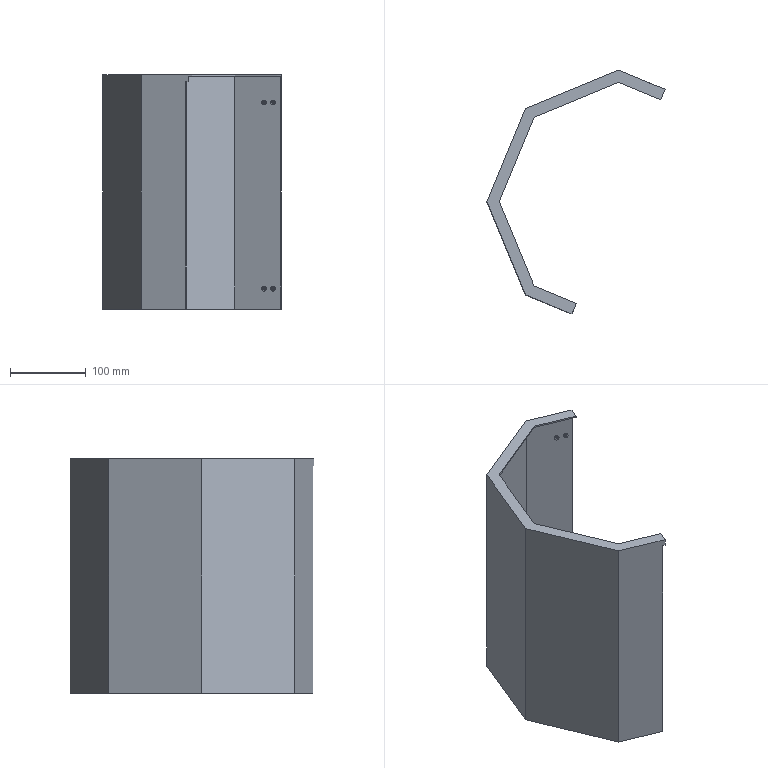Part | SolidWorks | features ICE 4, Extrusion 1, HoleWzd 1, RefAxis 1, Shell 1 | 1 solid | 42 faces | box 235.877 x 323.01 x 310 mm | volume 339899 mm3 | plane 26 | cylinder 16 | commonest cylinder face diameters 2.5 x8 6 x8
STEP:
#1=CARTESIAN_POINT('',(37.476,154.412,26.75));
#2=VERTEX_POINT('',#1);
#3=CARTESIAN_POINT('',(39.786,153.456,26.75));
#4=VERTEX_POINT('',#3);
#5=CARTESIAN_POINT('',(38.631,153.934,26.75));
#6=DIRECTION('',(-0.3827,-0.9239,0.));
#7=DIRECTION('',(0.9239,-0.3827,0.));
#8=AXIS2_PLACEMENT_3D('',#5,#6,#7);
#9=CIRCLE('',#8,1.25);
#10=EDGE_CURVE('',#2,#4,#9,.T.);
#11=ORIENTED_EDGE('',*,*,#10,.T.);
#12=CARTESIAN_POINT('',(41.317,157.151,26.75));
#13=VERTEX_POINT('',#12);
#14=CARTESIAN_POINT('',(41.317,157.151,26.75));
#15=DIRECTION('',(0.3827,0.9239,0.));
#16=VECTOR('',#15,1000.);
#17=LINE('',#14,#16);
#18=EDGE_CURVE('',#4,#13,#17,.T.);
#19=ORIENTED_EDGE('',*,*,#18,.T.);
#20=CARTESIAN_POINT('',(39.007,158.108,26.75));
#21=VERTEX_POINT('',#20);
#22=CARTESIAN_POINT('',(40.162,157.63,26.75));
#23=DIRECTION('',(0.3827,0.9239,0.));
#24=DIRECTION('',(-0.9239,0.3827,0.));
#25=AXIS2_PLACEMENT_3D('',#22,#23,#24);
#26=CIRCLE('',#25,1.25);
#27=EDGE_CURVE('',#13,#21,#26,.T.);
#28=ORIENTED_EDGE('',*,*,#27,.T.);
#29=CARTESIAN_POINT('',(39.007,158.108,26.75));
#30=DIRECTION('',(0.3827,0.9239,0.));
#31=VECTOR('',#30,1000.);
#32=LINE('',#29,#31);
#33=EDGE_CURVE('',#2,#21,#32,.T.);
#34=ORIENTED_EDGE('',*,*,#33,.F.);
#35=EDGE_LOOP('',(#11,#19,#28,#34));
#36=FACE_OUTER_BOUND('',#35,.T.);
#37=CARTESIAN_POINT('',(40.162,157.63,26.75));
#38=DIRECTION('',(0.3827,0.9239,0.));
#39=DIRECTION('',(-0.9239,0.3827,0.));
#40=AXIS2_PLACEMENT_3D('',#37,#38,#39);
#41=CYLINDRICAL_SURFACE('',#40,1.25);
#42=ADVANCED_FACE('',(#36),#41,.F.);
#43=CARTESIAN_POINT('',(49.487,149.438,26.75));
#44=VERTEX_POINT('',#43);
#45=CARTESIAN_POINT('',(51.796,148.481,26.75));
#46=VERTEX_POINT('',#45);
#47=CARTESIAN_POINT('',(50.641,148.959,26.75));
#48=DIRECTION('',(-0.3827,-0.9239,0.));
#49=DIRECTION('',(0.9239,-0.3827,0.));
#50=AXIS2_PLACEMENT_3D('',#47,#48,#49);
#51=CIRCLE('',#50,1.25);
#52=EDGE_CURVE('',#44,#46,#51,.T.);
#53=ORIENTED_EDGE('',*,*,#52,.T.);
#54=CARTESIAN_POINT('',(53.327,152.176,26.75));
#55=VERTEX_POINT('',#54);
#56=CARTESIAN_POINT('',(53.327,152.176,26.75));
#57=DIRECTION('',(0.3827,0.9239,0.));
#58=VECTOR('',#57,1000.);
#59=LINE('',#56,#58);
#60=EDGE_CURVE('',#46,#55,#59,.T.);
#61=ORIENTED_EDGE('',*,*,#60,.T.);
#62=CARTESIAN_POINT('',(51.017,153.133,26.75));
#63=VERTEX_POINT('',#62);
#64=CARTESIAN_POINT('',(52.172,152.655,26.75));
#65=DIRECTION('',(0.3827,0.9239,0.));
#66=DIRECTION('',(-0.9239,0.3827,0.));
#67=AXIS2_PLACEMENT_3D('',#64,#65,#66);
#68=CIRCLE('',#67,1.25);
#69=EDGE_CURVE('',#55,#63,#68,.T.);
#70=ORIENTED_EDGE('',*,*,#69,.T.);
#71=CARTESIAN_POINT('',(51.017,153.133,26.75));
#72=DIRECTION('',(0.3827,0.9239,0.));
#73=VECTOR('',#72,1000.);
#74=LINE('',#71,#73);
#75=EDGE_CURVE('',#44,#63,#74,.T.);
#76=ORIENTED_EDGE('',*,*,#75,.F.);
#77=EDGE_LOOP('',(#53,#61,#70,#76));
#78=FACE_OUTER_BOUND('',#77,.T.);
#79=CARTESIAN_POINT('',(52.172,152.655,26.75));
#80=DIRECTION('',(0.3827,0.9239,0.));
#81=DIRECTION('',(-0.9239,0.3827,0.));
#82=AXIS2_PLACEMENT_3D('',#79,#80,#81);
#83=CYLINDRICAL_SURFACE('',#82,1.25);
#84=ADVANCED_FACE('',(#78),#83,.F.);
#85=CARTESIAN_POINT('',(37.476,154.412,273.25));
#86=VERTEX_POINT('',#85);
#87=CARTESIAN_POINT('',(39.786,153.456,273.25));
#88=VERTEX_POINT('',#87);
#89=CARTESIAN_POINT('',(38.631,153.934,273.25));
#90=DIRECTION('',(-0.3827,-0.9239,0.));
#91=DIRECTION('',(0.9239,-0.3827,0.));
#92=AXIS2_PLACEMENT_3D('',#89,#90,#91);
#93=CIRCLE('',#92,1.25);
#94=EDGE_CURVE('',#86,#88,#93,.T.);
#95=ORIENTED_EDGE('',*,*,#94,.T.);
#96=CARTESIAN_POINT('',(41.317,157.151,273.25));
#97=VERTEX_POINT('',#96);
#98=CARTESIAN_POINT('',(41.317,157.151,273.25));
#99=DIRECTION('',(0.3827,0.9239,0.));
#100=VECTOR('',#99,1000.);
#101=LINE('',#98,#100);
#102=EDGE_CURVE('',#88,#97,#101,.T.);
#103=ORIENTED_EDGE('',*,*,#102,.T.);
#104=CARTESIAN_POINT('',(39.007,158.108,273.25));
#105=VERTEX_POINT('',#104);
#106=CARTESIAN_POINT('',(40.162,157.63,273.25));
#107=DIRECTION('',(0.3827,0.9239,0.));
#108=DIRECTION('',(-0.9239,0.3827,0.));
#109=AXIS2_PLACEMENT_3D('',#106,#107,#108);
#110=CIRCLE('',#109,1.25);
#111=EDGE_CURVE('',#97,#105,#110,.T.);
#112=ORIENTED_EDGE('',*,*,#111,.T.);
#113=CARTESIAN_POINT('',(39.007,158.108,273.25));
#114=DIRECTION('',(0.3827,0.9239,0.));
#115=VECTOR('',#114,1000.);
#116=LINE('',#113,#115);
#117=EDGE_CURVE('',#86,#105,#116,.T.);
#118=ORIENTED_EDGE('',*,*,#117,.F.);
#119=EDGE_LOOP('',(#95,#103,#112,#118));
#120=FACE_OUTER_BOUND('',#119,.T.);
#121=CARTESIAN_POINT('',(40.162,157.63,273.25));
#122=DIRECTION('',(0.3827,0.9239,0.));
#123=DIRECTION('',(-0.9239,0.3827,0.));
#124=AXIS2_PLACEMENT_3D('',#121,#122,#123);
#125=CYLINDRICAL_SURFACE('',#124,1.25);
#126=ADVANCED_FACE('',(#120),#125,.F.);
#127=CARTESIAN_POINT('',(49.487,149.438,273.25));
#128=VERTEX_POINT('',#127);
#129=CARTESIAN_POINT('',(51.796,148.481,273.25));
#130=VERTEX_POINT('',#129);
#131=CARTESIAN_POINT('',(50.641,148.959,273.25));
#132=DIRECTION('',(-0.3827,-0.9239,0.));
#133=DIRECTION('',(0.9239,-0.3827,0.));
#134=AXIS2_PLACEMENT_3D('',#131,#132,#133);
#135=CIRCLE('',#134,1.25);
#136=EDGE_CURVE('',#128,#130,#135,.T.);
#137=ORIENTED_EDGE('',*,*,#136,.T.);
#138=CARTESIAN_POINT('',(53.327,152.176,273.25));
#139=VERTEX_POINT('',#138);
#140=CARTESIAN_POINT('',(53.327,152.176,273.25));
#141=DIRECTION('',(0.3827,0.9239,0.));
#142=VECTOR('',#141,1000.);
#143=LINE('',#140,#142);
#144=EDGE_CURVE('',#130,#139,#143,.T.);
#145=ORIENTED_EDGE('',*,*,#144,.T.);
#146=CARTESIAN_POINT('',(51.017,153.133,273.25));
#147=VERTEX_POINT('',#146);
#148=CARTESIAN_POINT('',(52.172,152.655,273.25));
#149=DIRECTION('',(0.3827,0.9239,0.));
#150=DIRECTION('',(-0.9239,0.3827,0.));
#151=AXIS2_PLACEMENT_3D('',#148,#149,#150);
#152=CIRCLE('',#151,1.25);
#153=EDGE_CURVE('',#139,#147,#152,.T.);
#154=ORIENTED_EDGE('',*,*,#153,.T.);
#155=CARTESIAN_POINT('',(51.017,153.133,273.25));
#156=DIRECTION('',(0.3827,0.9239,0.));
#157=VECTOR('',#156,1000.);
#158=LINE('',#155,#157);
#159=EDGE_CURVE('',#128,#147,#158,.T.);
#160=ORIENTED_EDGE('',*,*,#159,.F.);
#161=EDGE_LOOP('',(#137,#145,#154,#160));
#162=FACE_OUTER_BOUND('',#161,.T.);
#163=CARTESIAN_POINT('',(52.172,152.655,273.25));
#164=DIRECTION('',(0.3827,0.9239,0.));
#165=DIRECTION('',(-0.9239,0.3827,0.));
#166=AXIS2_PLACEMENT_3D('',#163,#164,#165);
#167=CYLINDRICAL_SURFACE('',#166,1.25);
#168=ADVANCED_FACE('',(#162),#167,.F.);
#169=CARTESIAN_POINT('',(41.403,152.786,26.75));
#170=VERTEX_POINT('',#169);
#171=CARTESIAN_POINT('',(35.859,155.082,26.75));
#172=VERTEX_POINT('',#171);
#173=CARTESIAN_POINT('',(38.631,153.934,26.75));
#174=DIRECTION('',(-0.3827,-0.9239,0.));
#175=DIRECTION('',(0.9239,-0.3827,0.));
#176=AXIS2_PLACEMENT_3D('',#173,#174,#175);
#177=CIRCLE('',#176,3.);
#178=EDGE_CURVE('',#170,#172,#177,.T.);
#179=ORIENTED_EDGE('',*,*,#178,.F.);
#180=CARTESIAN_POINT('',(42.168,154.634,26.75));
#181=VERTEX_POINT('',#180);
#182=CARTESIAN_POINT('',(41.403,152.786,26.75));
#183=DIRECTION('',(0.3827,0.9239,0.));
#184=VECTOR('',#183,1000.);
#185=LINE('',#182,#184);
#186=EDGE_CURVE('',#170,#181,#185,.T.);
#187=ORIENTED_EDGE('',*,*,#186,.T.);
#188=CARTESIAN_POINT('',(36.625,156.93,26.75));
#189=VERTEX_POINT('',#188);
#190=CARTESIAN_POINT('',(39.396,155.782,26.75));
#191=DIRECTION('',(-0.3827,-0.9239,0.));
#192=DIRECTION('',(0.9239,-0.3827,0.));
#193=AXIS2_PLACEMENT_3D('',#190,#191,#192);
#194=CIRCLE('',#193,3.);
#195=EDGE_CURVE('',#181,#189,#194,.T.);
#196=ORIENTED_EDGE('',*,*,#195,.T.);
#197=CARTESIAN_POINT('',(35.859,155.082,26.75));
#198=DIRECTION('',(0.3827,0.9239,0.));
#199=VECTOR('',#198,1000.);
#200=LINE('',#197,#199);
#201=EDGE_CURVE('',#172,#189,#200,.T.);
#202=ORIENTED_EDGE('',*,*,#201,.F.);
#203=EDGE_LOOP('',(#179,#187,#196,#202));
#204=FACE_OUTER_BOUND('',#203,.T.);
#205=CARTESIAN_POINT('',(38.631,153.934,26.75));
#206=DIRECTION('',(0.3827,0.9239,0.));
#207=DIRECTION('',(-0.9239,0.3827,0.));
#208=AXIS2_PLACEMENT_3D('',#205,#206,#207);
#209=CYLINDRICAL_SURFACE('',#208,3.);
#210=ADVANCED_FACE('',(#204),#209,.T.);
#211=CARTESIAN_POINT('',(53.413,147.811,26.75));
#212=VERTEX_POINT('',#211);
#213=CARTESIAN_POINT('',(47.87,150.107,26.75));
#214=VERTEX_POINT('',#213);
#215=CARTESIAN_POINT('',(50.641,148.959,26.75));
#216=DIRECTION('',(-0.3827,-0.9239,0.));
#217=DIRECTION('',(0.9239,-0.3827,0.));
#218=AXIS2_PLACEMENT_3D('',#215,#216,#217);
#219=CIRCLE('',#218,3.);
#220=EDGE_CURVE('',#212,#214,#219,.T.);
#221=ORIENTED_EDGE('',*,*,#220,.F.);
#222=CARTESIAN_POINT('',(54.178,149.659,26.75));
#223=VERTEX_POINT('',#222);
#224=CARTESIAN_POINT('',(53.413,147.811,26.75));
#225=DIRECTION('',(0.3827,0.9239,0.));
#226=VECTOR('',#225,1000.);
#227=LINE('',#224,#226);
#228=EDGE_CURVE('',#212,#223,#227,.T.);
#229=ORIENTED_EDGE('',*,*,#228,.T.);
#230=CARTESIAN_POINT('',(48.635,151.955,26.75));
#231=VERTEX_POINT('',#230);
#232=CARTESIAN_POINT('',(51.407,150.807,26.75));
#233=DIRECTION('',(-0.3827,-0.9239,0.));
#234=DIRECTION('',(0.9239,-0.3827,0.));
#235=AXIS2_PLACEMENT_3D('',#232,#233,#234);
#236=CIRCLE('',#235,3.);
#237=EDGE_CURVE('',#223,#231,#236,.T.);
#238=ORIENTED_EDGE('',*,*,#237,.T.);
#239=CARTESIAN_POINT('',(47.87,150.107,26.75));
#240=DIRECTION('',(0.3827,0.9239,0.));
#241=VECTOR('',#240,1000.);
#242=LINE('',#239,#241);
#243=EDGE_CURVE('',#214,#231,#242,.T.);
#244=ORIENTED_EDGE('',*,*,#243,.F.);
#245=EDGE_LOOP('',(#221,#229,#238,#244));
#246=FACE_OUTER_BOUND('',#245,.T.);
#247=CARTESIAN_POINT('',(50.641,148.959,26.75));
#248=DIRECTION('',(0.3827,0.9239,0.));
#249=DIRECTION('',(-0.9239,0.3827,0.));
#250=AXIS2_PLACEMENT_3D('',#247,#248,#249);
#251=CYLINDRICAL_SURFACE('',#250,3.);
#252=ADVANCED_FACE('',(#246),#251,.T.);
#253=CARTESIAN_POINT('',(53.413,147.811,273.25));
#254=VERTEX_POINT('',#253);
#255=CARTESIAN_POINT('',(47.87,150.107,273.25));
#256=VERTEX_POINT('',#255);
#257=CARTESIAN_POINT('',(50.641,148.959,273.25));
#258=DIRECTION('',(-0.3827,-0.9239,0.));
#259=DIRECTION('',(0.9239,-0.3827,0.));
#260=AXIS2_PLACEMENT_3D('',#257,#258,#259);
#261=CIRCLE('',#260,3.);
#262=EDGE_CURVE('',#254,#256,#261,.T.);
#263=ORIENTED_EDGE('',*,*,#262,.F.);
#264=CARTESIAN_POINT('',(54.178,149.659,273.25));
#265=VERTEX_POINT('',#264);
#266=CARTESIAN_POINT('',(53.413,147.811,273.25));
#267=DIRECTION('',(0.3827,0.9239,0.));
#268=VECTOR('',#267,1000.);
#269=LINE('',#266,#268);
#270=EDGE_CURVE('',#254,#265,#269,.T.);
#271=ORIENTED_EDGE('',*,*,#270,.T.);
#272=CARTESIAN_POINT('',(48.635,151.955,273.25));
#273=VERTEX_POINT('',#272);
#274=CARTESIAN_POINT('',(51.407,150.807,273.25));
#275=DIRECTION('',(-0.3827,-0.9239,0.));
#276=DIRECTION('',(0.9239,-0.3827,0.));
#277=AXIS2_PLACEMENT_3D('',#274,#275,#276);
#278=CIRCLE('',#277,3.);
#279=EDGE_CURVE('',#265,#273,#278,.T.);
#280=ORIENTED_EDGE('',*,*,#279,.T.);
#281=CARTESIAN_POINT('',(47.87,150.107,273.25));
#282=DIRECTION('',(0.3827,0.9239,0.));
#283=VECTOR('',#282,1000.);
#284=LINE('',#281,#283);
#285=EDGE_CURVE('',#256,#273,#284,.T.);
#286=ORIENTED_EDGE('',*,*,#285,.F.);
#287=EDGE_LOOP('',(#263,#271,#280,#286));
#288=FACE_OUTER_BOUND('',#287,.T.);
#289=CARTESIAN_POINT('',(50.641,148.959,273.25));
#290=DIRECTION('',(0.3827,0.9239,0.));
#291=DIRECTION('',(-0.9239,0.3827,0.));
#292=AXIS2_PLACEMENT_3D('',#289,#290,#291);
#293=CYLINDRICAL_SURFACE('',#292,3.);
#294=ADVANCED_FACE('',(#288),#293,.T.);
#295=CARTESIAN_POINT('',(41.403,152.786,273.25));
#296=VERTEX_POINT('',#295);
#297=CARTESIAN_POINT('',(35.859,155.082,273.25));
#298=VERTEX_POINT('',#297);
#299=CARTESIAN_POINT('',(38.631,153.934,273.25));
#300=DIRECTION('',(-0.3827,-0.9239,0.));
#301=DIRECTION('',(0.9239,-0.3827,0.));
#302=AXIS2_PLACEMENT_3D('',#299,#300,#301);
#303=CIRCLE('',#302,3.);
#304=EDGE_CURVE('',#296,#298,#303,.T.);
#305=ORIENTED_EDGE('',*,*,#304,.F.);
#306=CARTESIAN_POINT('',(42.168,154.634,273.25));
#307=VERTEX_POINT('',#306);
#308=CARTESIAN_POINT('',(41.403,152.786,273.25));
#309=DIRECTION('',(0.3827,0.9239,0.));
#310=VECTOR('',#309,1000.);
#311=LINE('',#308,#310);
#312=EDGE_CURVE('',#296,#307,#311,.T.);
#313=ORIENTED_EDGE('',*,*,#312,.T.);
#314=CARTESIAN_POINT('',(36.625,156.93,273.25));
#315=VERTEX_POINT('',#314);
#316=CARTESIAN_POINT('',(39.396,155.782,273.25));
#317=DIRECTION('',(-0.3827,-0.9239,0.));
#318=DIRECTION('',(0.9239,-0.3827,0.));
#319=AXIS2_PLACEMENT_3D('',#316,#317,#318);
#320=CIRCLE('',#319,3.);
#321=EDGE_CURVE('',#307,#315,#320,.T.);
#322=ORIENTED_EDGE('',*,*,#321,.T.);
#323=CARTESIAN_POINT('',(35.859,155.082,273.25));
#324=DIRECTION('',(0.3827,0.9239,0.));
#325=VECTOR('',#324,1000.);
#326=LINE('',#323,#325);
#327=EDGE_CURVE('',#298,#315,#326,.T.);
#328=ORIENTED_EDGE('',*,*,#327,.F.);
#329=EDGE_LOOP('',(#305,#313,#322,#328));
#330=FACE_OUTER_BOUND('',#329,.T.);
#331=CARTESIAN_POINT('',(38.631,153.934,273.25));
#332=DIRECTION('',(0.3827,0.9239,0.));
#333=DIRECTION('',(-0.9239,0.3827,0.));
#334=AXIS2_PLACEMENT_3D('',#331,#332,#333);
#335=CYLINDRICAL_SURFACE('',#334,3.);
#336=ADVANCED_FACE('',(#330),#335,.T.);
#337=CARTESIAN_POINT('',(51.407,150.807,26.75));
#338=DIRECTION('',(-0.3827,-0.9239,0.));
#339=DIRECTION('',(0.9239,-0.3827,0.));
#340=AXIS2_PLACEMENT_3D('',#337,#338,#339);
#341=CIRCLE('',#340,3.);
#342=EDGE_CURVE('',#231,#223,#341,.T.);
#343=ORIENTED_EDGE('',*,*,#342,.F.);
#344=ORIENTED_EDGE('',*,*,#237,.F.);
#345=EDGE_LOOP('',(#343,#344));
#346=FACE_BOUND('',#345,.T.);
#347=CARTESIAN_POINT('',(39.396,155.782,273.25));
#348=DIRECTION('',(-0.3827,-0.9239,0.));
#349=DIRECTION('',(0.9239,-0.3827,0.));
#350=AXIS2_PLACEMENT_3D('',#347,#348,#349);
#351=CIRCLE('',#350,3.);
#352=EDGE_CURVE('',#315,#307,#351,.T.);
#353=ORIENTED_EDGE('',*,*,#352,.F.);
#354=ORIENTED_EDGE('',*,*,#321,.F.);
#355=EDGE_LOOP('',(#353,#354));
#356=FACE_BOUND('',#355,.T.);
#357=CARTESIAN_POINT('',(60.847,146.897,308.));
#358=VERTEX_POINT('',#357);
#359=CARTESIAN_POINT('',(60.847,146.897,0.));
#360=VERTEX_POINT('',#359);
#361=CARTESIAN_POINT('',(60.847,146.897,310.));
#362=DIRECTION('',(0.,0.,-1.));
#363=VECTOR('',#362,1000.);
#364=LINE('',#361,#363);
#365=EDGE_CURVE('',#358,#360,#364,.T.);
#366=ORIENTED_EDGE('',*,*,#365,.F.);
#367=CARTESIAN_POINT('',(0.,172.1,308.));
#368=VERTEX_POINT('',#367);
#369=CARTESIAN_POINT('',(122.459,121.376,308.));
#370=DIRECTION('',(-0.9239,0.3827,0.));
#371=VECTOR('',#370,1000.);
#372=LINE('',#369,#371);
#373=EDGE_CURVE('',#358,#368,#372,.T.);
#374=ORIENTED_EDGE('',*,*,#373,.T.);
#375=CARTESIAN_POINT('',(0.,172.1,0.));
#376=VERTEX_POINT('',#375);
#377=CARTESIAN_POINT('',(0.,172.1,310.));
#378=DIRECTION('',(0.,0.,-1.));
#379=VECTOR('',#378,1000.);
#380=LINE('',#377,#379);
#381=EDGE_CURVE('',#368,#376,#380,.T.);
#382=ORIENTED_EDGE('',*,*,#381,.T.);
#383=CARTESIAN_POINT('',(122.459,121.376,0.));
#384=DIRECTION('',(-0.9239,0.3827,0.));
#385=VECTOR('',#384,1000.);
#386=LINE('',#383,#385);
#387=EDGE_CURVE('',#360,#376,#386,.T.);
#388=ORIENTED_EDGE('',*,*,#387,.F.);
#389=EDGE_LOOP('',(#366,#374,#382,#388));
#390=FACE_OUTER_BOUND('',#389,.T.);
#391=CARTESIAN_POINT('',(51.407,150.807,273.25));
#392=DIRECTION('',(-0.3827,-0.9239,0.));
#393=DIRECTION('',(0.9239,-0.3827,0.));
#394=AXIS2_PLACEMENT_3D('',#391,#392,#393);
#395=CIRCLE('',#394,3.);
#396=EDGE_CURVE('',#273,#265,#395,.T.);
#397=ORIENTED_EDGE('',*,*,#396,.F.);
#398=ORIENTED_EDGE('',*,*,#279,.F.);
#399=EDGE_LOOP('',(#397,#398));
#400=FACE_BOUND('',#399,.T.);
#401=CARTESIAN_POINT('',(39.396,155.782,26.75));
#402=DIRECTION('',(-0.3827,-0.9239,0.));
#403=DIRECTION('',(0.9239,-0.3827,0.));
#404=AXIS2_PLACEMENT_3D('',#401,#402,#403);
#405=CIRCLE('',#404,3.);
#406=EDGE_CURVE('',#189,#181,#405,.T.);
#407=ORIENTED_EDGE('',*,*,#406,.F.);
#408=ORIENTED_EDGE('',*,*,#195,.F.);
#409=EDGE_LOOP('',(#407,#408));
#410=FACE_BOUND('',#409,.T.);
#411=CARTESIAN_POINT('',(122.459,121.376,310.));
#412=DIRECTION('',(-0.3827,-0.9239,0.));
#413=DIRECTION('',(0.9239,-0.3827,0.));
#414=AXIS2_PLACEMENT_3D('',#411,#412,#413);
#415=PLANE('',#414);
#416=ADVANCED_FACE('',(#346,#356,#390,#400,#410),#415,.T.);
#417=CARTESIAN_POINT('',(-64.846,-147.405,301.));
#418=VERTEX_POINT('',#417);
#419=CARTESIAN_POINT('',(-64.846,-147.405,0.));
#420=VERTEX_POINT('',#419);
#421=CARTESIAN_POINT('',(-64.846,-147.405,0.));
#422=DIRECTION('',(0.,0.,-1.));
#423=VECTOR('',#422,1000.);
#424=LINE('',#421,#423);
#425=EDGE_CURVE('',#418,#420,#424,.T.);
#426=ORIENTED_EDGE('',*,*,#425,.F.);
#427=CARTESIAN_POINT('',(-61.612,-148.745,301.));
#428=VERTEX_POINT('',#427);
#429=CARTESIAN_POINT('',(-61.612,-148.745,301.));
#430=DIRECTION('',(-0.9239,0.3827,0.));
#431=VECTOR('',#430,1000.);
#432=LINE('',#429,#431);
#433=EDGE_CURVE('',#428,#418,#432,.T.);
#434=ORIENTED_EDGE('',*,*,#433,.F.);
#435=CARTESIAN_POINT('',(-61.612,-148.745,310.));
#436=VERTEX_POINT('',#435);
#437=CARTESIAN_POINT('',(-61.612,-148.745,310.));
#438=DIRECTION('',(0.,0.,1.));
#439=VECTOR('',#438,1000.);
#440=LINE('',#437,#439);
#441=EDGE_CURVE('',#428,#436,#440,.T.);
#442=ORIENTED_EDGE('',*,*,#441,.T.);
#443=CARTESIAN_POINT('',(-123.224,-123.224,310.));
#444=VERTEX_POINT('',#443);
#445=CARTESIAN_POINT('',(-123.224,-123.224,310.));
#446=DIRECTION('',(0.9239,-0.3827,0.));
#447=VECTOR('',#446,1000.);
#448=LINE('',#445,#447);
#449=EDGE_CURVE('',#444,#436,#448,.T.);
#450=ORIENTED_EDGE('',*,*,#449,.F.);
#451=CARTESIAN_POINT('',(-123.224,-123.224,0.));
#452=VERTEX_POINT('',#451);
#453=CARTESIAN_POINT('',(-123.224,-123.224,310.));
#454=DIRECTION('',(0.,0.,-1.));
#455=VECTOR('',#454,1000.);
#456=LINE('',#453,#455);
#457=EDGE_CURVE('',#444,#452,#456,.T.);
#458=ORIENTED_EDGE('',*,*,#457,.T.);
#459=CARTESIAN_POINT('',(-123.224,-123.224,0.));
#460=DIRECTION('',(0.9239,-0.3827,0.));
#461=VECTOR('',#460,1000.);
#462=LINE('',#459,#461);
#463=EDGE_CURVE('',#452,#420,#462,.T.);
#464=ORIENTED_EDGE('',*,*,#463,.T.);
#465=EDGE_LOOP('',(#426,#434,#442,#450,#458,#464));
#466=FACE_OUTER_BOUND('',#465,.T.);
#467=CARTESIAN_POINT('',(-123.224,-123.224,310.));
#468=DIRECTION('',(0.3827,0.9239,0.));
#469=DIRECTION('',(-0.9239,0.3827,0.));
#470=AXIS2_PLACEMENT_3D('',#467,#468,#469);
#471=PLANE('',#470);
#472=ADVANCED_FACE('',(#466),#471,.F.);
#473=CARTESIAN_POINT('',(40.162,157.63,26.75));
#474=DIRECTION('',(0.3827,0.9239,0.));
#475=DIRECTION('',(-0.9239,0.3827,0.));
#476=AXIS2_PLACEMENT_3D('',#473,#474,#475);
#477=CIRCLE('',#476,1.25);
#478=EDGE_CURVE('',#21,#13,#477,.T.);
#479=ORIENTED_EDGE('',*,*,#478,.F.);
#480=ORIENTED_EDGE('',*,*,#27,.F.);
#481=EDGE_LOOP('',(#479,#480));
#482=FACE_BOUND('',#481,.T.);
#483=CARTESIAN_POINT('',(52.172,152.655,26.75));
#484=DIRECTION('',(0.3827,0.9239,0.));
#485=DIRECTION('',(-0.9239,0.3827,0.));
#486=AXIS2_PLACEMENT_3D('',#483,#484,#485);
#487=CIRCLE('',#486,1.25);
#488=EDGE_CURVE('',#63,#55,#487,.T.);
#489=ORIENTED_EDGE('',*,*,#488,.F.);
#490=ORIENTED_EDGE('',*,*,#69,.F.);
#491=EDGE_LOOP('',(#489,#490));
#492=FACE_BOUND('',#491,.T.);
#493=CARTESIAN_POINT('',(40.162,157.63,273.25));
#494=DIRECTION('',(0.3827,0.9239,0.));
#495=DIRECTION('',(-0.9239,0.3827,0.));
#496=AXIS2_PLACEMENT_3D('',#493,#494,#495);
#497=CIRCLE('',#496,1.25);
#498=EDGE_CURVE('',#105,#97,#497,.T.);
#499=ORIENTED_EDGE('',*,*,#498,.F.);
#500=ORIENTED_EDGE('',*,*,#111,.F.);
#501=EDGE_LOOP('',(#499,#500));
#502=FACE_BOUND('',#501,.T.);
#503=CARTESIAN_POINT('',(52.172,152.655,273.25));
#504=DIRECTION('',(0.3827,0.9239,0.));
#505=DIRECTION('',(-0.9239,0.3827,0.));
#506=AXIS2_PLACEMENT_3D('',#503,#504,#505);
#507=CIRCLE('',#506,1.25);
#508=EDGE_CURVE('',#147,#139,#507,.T.);
#509=ORIENTED_EDGE('',*,*,#508,.F.);
#510=ORIENTED_EDGE('',*,*,#153,.F.);
#511=EDGE_LOOP('',(#509,#510));
#512=FACE_BOUND('',#511,.T.);
#513=CARTESIAN_POINT('',(61.612,148.745,310.));
#514=VERTEX_POINT('',#513);
#515=CARTESIAN_POINT('',(0.,174.265,310.));
#516=VERTEX_POINT('',#515);
#517=CARTESIAN_POINT('',(123.224,123.224,310.));
#518=DIRECTION('',(-0.9239,0.3827,0.));
#519=VECTOR('',#518,1000.);
#520=LINE('',#517,#519);
#521=EDGE_CURVE('',#514,#516,#520,.T.);
#522=ORIENTED_EDGE('',*,*,#521,.F.);
#523=CARTESIAN_POINT('',(61.612,148.745,0.));
#524=VERTEX_POINT('',#523);
#525=CARTESIAN_POINT('',(61.612,148.745,310.));
#526=DIRECTION('',(0.,0.,-1.));
#527=VECTOR('',#526,1000.);
#528=LINE('',#525,#527);
#529=EDGE_CURVE('',#514,#524,#528,.T.);
#530=ORIENTED_EDGE('',*,*,#529,.T.);
#531=CARTESIAN_POINT('',(0.,174.265,0.));
#532=VERTEX_POINT('',#531);
#533=CARTESIAN_POINT('',(123.224,123.224,0.));
#534=DIRECTION('',(-0.9239,0.3827,0.));
#535=VECTOR('',#534,1000.);
#536=LINE('',#533,#535);
#537=EDGE_CURVE('',#524,#532,#536,.T.);
#538=ORIENTED_EDGE('',*,*,#537,.T.);
#539=CARTESIAN_POINT('',(0.,174.265,310.));
#540=DIRECTION('',(0.,0.,-1.));
#541=VECTOR('',#540,1000.);
#542=LINE('',#539,#541);
#543=EDGE_CURVE('',#516,#532,#542,.T.);
#544=ORIENTED_EDGE('',*,*,#543,.F.);
#545=EDGE_LOOP('',(#522,#530,#538,#544));
#546=FACE_OUTER_BOUND('',#545,.T.);
#547=CARTESIAN_POINT('',(123.224,123.224,310.));
#548=DIRECTION('',(-0.3827,-0.9239,0.));
#549=DIRECTION('',(0.9239,-0.3827,0.));
#550=AXIS2_PLACEMENT_3D('',#547,#548,#549);
#551=PLANE('',#550);
#552=ADVANCED_FACE('',(#482,#492,#502,#512,#546),#551,.F.);
#553=CARTESIAN_POINT('',(-123.224,123.224,0.));
#554=VERTEX_POINT('',#553);
#555=CARTESIAN_POINT('',(0.,174.265,0.));
#556=DIRECTION('',(-0.9239,-0.3827,0.));
#557=VECTOR('',#556,1000.);
#558=LINE('',#555,#557);
#559=EDGE_CURVE('',#532,#554,#558,.T.);
#560=ORIENTED_EDGE('',*,*,#559,.T.);
#561=CARTESIAN_POINT('',(-123.224,123.224,310.));
#562=VERTEX_POINT('',#561);
#563=CARTESIAN_POINT('',(-123.224,123.224,310.));
#564=DIRECTION('',(0.,0.,-1.));
#565=VECTOR('',#564,1000.);
#566=LINE('',#563,#565);
#567=EDGE_CURVE('',#562,#554,#566,.T.);
#568=ORIENTED_EDGE('',*,*,#567,.F.);
#569=CARTESIAN_POINT('',(0.,174.265,310.));
#570=DIRECTION('',(-0.9239,-0.3827,0.));
#571=VECTOR('',#570,1000.);
#572=LINE('',#569,#571);
#573=EDGE_CURVE('',#516,#562,#572,.T.);
#574=ORIENTED_EDGE('',*,*,#573,.F.);
#575=ORIENTED_EDGE('',*,*,#543,.T.);
#576=EDGE_LOOP('',(#560,#568,#574,#575));
#577=FACE_OUTER_BOUND('',#576,.T.);
#578=CARTESIAN_POINT('',(0.,174.265,310.));
#579=DIRECTION('',(0.3827,-0.9239,0.));
#580=DIRECTION('',(0.9239,0.3827,0.));
#581=AXIS2_PLACEMENT_3D('',#578,#579,#580);
#582=PLANE('',#581);
#583=ADVANCED_FACE('',(#577),#582,.F.);
#584=CARTESIAN_POINT('',(-174.265,0.,0.));
#585=VERTEX_POINT('',#584);
#586=CARTESIAN_POINT('',(-123.224,123.224,0.));
#587=DIRECTION('',(-0.3827,-0.9239,0.));
#588=VECTOR('',#587,1000.);
#589=LINE('',#586,#588);
#590=EDGE_CURVE('',#554,#585,#589,.T.);
#591=ORIENTED_EDGE('',*,*,#590,.T.);
#592=CARTESIAN_POINT('',(-174.265,0.,310.));
#593=VERTEX_POINT('',#592);
#594=CARTESIAN_POINT('',(-174.265,0.,310.));
#595=DIRECTION('',(0.,0.,-1.));
#596=VECTOR('',#595,1000.);
#597=LINE('',#594,#596);
#598=EDGE_CURVE('',#593,#585,#597,.T.);
#599=ORIENTED_EDGE('',*,*,#598,.F.);
#600=CARTESIAN_POINT('',(-123.224,123.224,310.));
#601=DIRECTION('',(-0.3827,-0.9239,0.));
#602=VECTOR('',#601,1000.);
#603=LINE('',#600,#602);
#604=EDGE_CURVE('',#562,#593,#603,.T.);
#605=ORIENTED_EDGE('',*,*,#604,.F.);
#606=ORIENTED_EDGE('',*,*,#567,.T.);
#607=EDGE_LOOP('',(#591,#599,#605,#606));
#608=FACE_OUTER_BOUND('',#607,.T.);
#609=CARTESIAN_POINT('',(-123.224,123.224,310.));
#610=DIRECTION('',(0.9239,-0.3827,0.));
#611=DIRECTION('',(0.3827,0.9239,0.));
#612=AXIS2_PLACEMENT_3D('',#609,#610,#611);
#613=PLANE('',#612);
#614=ADVANCED_FACE('',(#608),#613,.F.);
#615=CARTESIAN_POINT('',(-174.265,0.,0.));
#616=DIRECTION('',(0.3827,-0.9239,0.));
#617=VECTOR('',#616,1000.);
#618=LINE('',#615,#617);
#619=EDGE_CURVE('',#585,#452,#618,.T.);
#620=ORIENTED_EDGE('',*,*,#619,.T.);
#621=ORIENTED_EDGE('',*,*,#457,.F.);
#622=CARTESIAN_POINT('',(-174.265,0.,310.));
#623=DIRECTION('',(0.3827,-0.9239,0.));
#624=VECTOR('',#623,1000.);
#625=LINE('',#622,#624);
#626=EDGE_CURVE('',#593,#444,#625,.T.);
#627=ORIENTED_EDGE('',*,*,#626,.F.);
#628=ORIENTED_EDGE('',*,*,#598,.T.);
#629=EDGE_LOOP('',(#620,#621,#627,#628));
#630=FACE_OUTER_BOUND('',#629,.T.);
#631=CARTESIAN_POINT('',(-174.265,0.,310.));
#632=DIRECTION('',(0.9239,0.3827,0.));
#633=DIRECTION('',(-0.3827,0.9239,0.));
#634=AXIS2_PLACEMENT_3D('',#631,#632,#633);
#635=PLANE('',#634);
#636=ADVANCED_FACE('',(#630),#635,.F.);
#637=CARTESIAN_POINT('',(55.872,134.886,310.));
#638=VERTEX_POINT('',#637);
#639=CARTESIAN_POINT('',(70.138,169.329,310.));
#640=DIRECTION('',(-0.3827,-0.9239,0.));
#641=VECTOR('',#640,1000.);
#642=LINE('',#639,#641);
#643=EDGE_CURVE('',#514,#638,#642,.T.);
#644=ORIENTED_EDGE('',*,*,#643,.F.);
#645=ORIENTED_EDGE('',*,*,#521,.T.);
#646=ORIENTED_EDGE('',*,*,#573,.T.);
#647=ORIENTED_EDGE('',*,*,#604,.T.);
#648=ORIENTED_EDGE('',*,*,#626,.T.);
#649=ORIENTED_EDGE('',*,*,#449,.T.);
#650=CARTESIAN_POINT('',(-55.872,-134.886,310.));
#651=VERTEX_POINT('',#650);
#652=CARTESIAN_POINT('',(70.138,169.329,310.));
#653=DIRECTION('',(-0.3827,-0.9239,0.));
#654=VECTOR('',#653,1000.);
#655=LINE('',#652,#654);
#656=EDGE_CURVE('',#651,#436,#655,.T.);
#657=ORIENTED_EDGE('',*,*,#656,.F.);
#658=CARTESIAN_POINT('',(-111.744,-111.744,310.));
#659=VERTEX_POINT('',#658);
#660=CARTESIAN_POINT('',(-111.744,-111.744,310.));
#661=DIRECTION('',(0.9239,-0.3827,0.));
#662=VECTOR('',#661,1000.);
#663=LINE('',#660,#662);
#664=EDGE_CURVE('',#659,#651,#663,.T.);
#665=ORIENTED_EDGE('',*,*,#664,.F.);
#666=CARTESIAN_POINT('',(-158.029,0.,310.));
#667=VERTEX_POINT('',#666);
#668=CARTESIAN_POINT('',(-158.029,0.,310.));
#669=DIRECTION('',(0.3827,-0.9239,0.));
#670=VECTOR('',#669,1000.);
#671=LINE('',#668,#670);
#672=EDGE_CURVE('',#667,#659,#671,.T.);
#673=ORIENTED_EDGE('',*,*,#672,.F.);
#674=CARTESIAN_POINT('',(-111.744,111.744,310.));
#675=VERTEX_POINT('',#674);
#676=CARTESIAN_POINT('',(-111.744,111.744,310.));
#677=DIRECTION('',(-0.3827,-0.9239,0.));
#678=VECTOR('',#677,1000.);
#679=LINE('',#676,#678);
#680=EDGE_CURVE('',#675,#667,#679,.T.);
#681=ORIENTED_EDGE('',*,*,#680,.F.);
#682=CARTESIAN_POINT('',(0.,158.029,310.));
#683=VERTEX_POINT('',#682);
#684=CARTESIAN_POINT('',(0.,158.029,310.));
#685=DIRECTION('',(-0.9239,-0.3827,0.));
#686=VECTOR('',#685,1000.);
#687=LINE('',#684,#686);
#688=EDGE_CURVE('',#683,#675,#687,.T.);
#689=ORIENTED_EDGE('',*,*,#688,.F.);
#690=CARTESIAN_POINT('',(111.744,111.744,310.));
#691=DIRECTION('',(-0.9239,0.3827,0.));
#692=VECTOR('',#691,1000.);
#693=LINE('',#690,#692);
#694=EDGE_CURVE('',#638,#683,#693,.T.);
#695=ORIENTED_EDGE('',*,*,#694,.F.);
#696=EDGE_LOOP('',(#644,#645,#646,#647,#648,#649,#657,#665,#673,#681,#689,#695));
#697=FACE_OUTER_BOUND('',#696,.T.);
#698=CARTESIAN_POINT('',(0.,0.,310.));
#699=DIRECTION('',(0.,0.,1.));
#700=DIRECTION('',(1.,0.,0.));
#701=AXIS2_PLACEMENT_3D('',#698,#699,#700);
#702=PLANE('',#701);
#703=ADVANCED_FACE('',(#697),#702,.T.);
#704=CARTESIAN_POINT('',(-121.693,-121.693,0.));
#705=VERTEX_POINT('',#704);
#706=CARTESIAN_POINT('',(-64.08,-145.557,0.));
#707=VERTEX_POINT('',#706);
#708=CARTESIAN_POINT('',(-122.459,-121.376,0.));
#709=DIRECTION('',(0.9239,-0.3827,0.));
#710=VECTOR('',#709,1000.);
#711=LINE('',#708,#710);
#712=EDGE_CURVE('',#705,#707,#711,.T.);
#713=ORIENTED_EDGE('',*,*,#712,.T.);
#714=CARTESIAN_POINT('',(67.402,171.868,0.));
#715=DIRECTION('',(-0.3827,-0.9239,0.));
#716=VECTOR('',#715,1000.);
#717=LINE('',#714,#716);
#718=EDGE_CURVE('',#707,#420,#717,.T.);
#719=ORIENTED_EDGE('',*,*,#718,.T.);
#720=ORIENTED_EDGE('',*,*,#463,.F.);
#721=ORIENTED_EDGE('',*,*,#619,.F.);
#722=ORIENTED_EDGE('',*,*,#590,.F.);
#723=ORIENTED_EDGE('',*,*,#559,.F.);
#724=ORIENTED_EDGE('',*,*,#537,.F.);
#725=CARTESIAN_POINT('',(70.138,169.329,0.));
#726=DIRECTION('',(-0.3827,-0.9239,0.));
#727=VECTOR('',#726,1000.);
#728=LINE('',#725,#727);
#729=EDGE_CURVE('',#524,#360,#728,.T.);
#730=ORIENTED_EDGE('',*,*,#729,.T.);
#731=ORIENTED_EDGE('',*,*,#387,.T.);
#732=CARTESIAN_POINT('',(-121.693,121.693,0.));
#733=VERTEX_POINT('',#732);
#734=CARTESIAN_POINT('',(0.7654,172.417,0.));
#735=DIRECTION('',(-0.9239,-0.3827,0.));
#736=VECTOR('',#735,1000.);
#737=LINE('',#734,#736);
#738=EDGE_CURVE('',#376,#733,#737,.T.);
#739=ORIENTED_EDGE('',*,*,#738,.T.);
#740=CARTESIAN_POINT('',(-172.1,0.,0.));
#741=VERTEX_POINT('',#740);
#742=CARTESIAN_POINT('',(-121.376,122.459,0.));
#743=DIRECTION('',(-0.3827,-0.9239,0.));
#744=VECTOR('',#743,1000.);
#745=LINE('',#742,#744);
#746=EDGE_CURVE('',#733,#741,#745,.T.);
#747=ORIENTED_EDGE('',*,*,#746,.T.);
#748=CARTESIAN_POINT('',(-172.417,0.7654,0.));
#749=DIRECTION('',(0.3827,-0.9239,0.));
#750=VECTOR('',#749,1000.);
#751=LINE('',#748,#750);
#752=EDGE_CURVE('',#741,#705,#751,.T.);
#753=ORIENTED_EDGE('',*,*,#752,.T.);
#754=EDGE_LOOP('',(#713,#719,#720,#721,#722,#723,#724,#730,#731,#739,#747,#753));
#755=FACE_OUTER_BOUND('',#754,.T.);
#756=CARTESIAN_POINT('',(0.,0.,0.));
#757=DIRECTION('',(0.,0.,1.));
#758=DIRECTION('',(1.,0.,0.));
#759=AXIS2_PLACEMENT_3D('',#756,#757,#758);
#760=PLANE('',#759);
#761=ADVANCED_FACE('',(#755),#760,.F.);
#762=CARTESIAN_POINT('',(-60.847,-146.897,301.));
#763=VERTEX_POINT('',#762);
#764=CARTESIAN_POINT('',(-64.08,-145.557,301.));
#765=VERTEX_POINT('',#764);
#766=CARTESIAN_POINT('',(-60.847,-146.897,301.));
#767=DIRECTION('',(-0.9239,0.3827,0.));
#768=VECTOR('',#767,1000.);
#769=LINE('',#766,#768);
#770=EDGE_CURVE('',#763,#765,#769,.T.);
#771=ORIENTED_EDGE('',*,*,#770,.T.);
#772=CARTESIAN_POINT('',(-64.08,-145.557,0.));
#773=DIRECTION('',(0.,0.,-1.));
#774=VECTOR('',#773,1000.);
#775=LINE('',#772,#774);
#776=EDGE_CURVE('',#765,#707,#775,.T.);
#777=ORIENTED_EDGE('',*,*,#776,.T.);
#778=ORIENTED_EDGE('',*,*,#712,.F.);
#779=CARTESIAN_POINT('',(-121.693,-121.693,308.));
#780=VERTEX_POINT('',#779);
#781=CARTESIAN_POINT('',(-121.693,-121.693,310.));
#782=DIRECTION('',(0.,0.,-1.));
#783=VECTOR('',#782,1000.);
#784=LINE('',#781,#783);
#785=EDGE_CURVE('',#780,#705,#784,.T.);
#786=ORIENTED_EDGE('',*,*,#785,.F.);
#787=CARTESIAN_POINT('',(-60.847,-146.897,308.));
#788=VERTEX_POINT('',#787);
#789=CARTESIAN_POINT('',(-122.459,-121.376,308.));
#790=DIRECTION('',(0.9239,-0.3827,0.));
#791=VECTOR('',#790,1000.);
#792=LINE('',#789,#791);
#793=EDGE_CURVE('',#780,#788,#792,.T.);
#794=ORIENTED_EDGE('',*,*,#793,.T.);
#795=CARTESIAN_POINT('',(-60.847,-146.897,310.));
#796=DIRECTION('',(0.,0.,1.));
#797=VECTOR('',#796,1000.);
#798=LINE('',#795,#797);
#799=EDGE_CURVE('',#763,#788,#798,.T.);
#800=ORIENTED_EDGE('',*,*,#799,.F.);
#801=EDGE_LOOP('',(#771,#777,#778,#786,#794,#800));
#802=FACE_OUTER_BOUND('',#801,.T.);
#803=CARTESIAN_POINT('',(-122.459,-121.376,310.));
#804=DIRECTION('',(0.3827,0.9239,0.));
#805=DIRECTION('',(-0.9239,0.3827,0.));
#806=AXIS2_PLACEMENT_3D('',#803,#804,#805);
#807=PLANE('',#806);
#808=ADVANCED_FACE('',(#802),#807,.T.);
#809=ORIENTED_EDGE('',*,*,#738,.F.);
#810=ORIENTED_EDGE('',*,*,#381,.F.);
#811=CARTESIAN_POINT('',(-121.693,121.693,308.));
#812=VERTEX_POINT('',#811);
#813=CARTESIAN_POINT('',(0.7654,172.417,308.));
#814=DIRECTION('',(-0.9239,-0.3827,0.));
#815=VECTOR('',#814,1000.);
#816=LINE('',#813,#815);
#817=EDGE_CURVE('',#368,#812,#816,.T.);
#818=ORIENTED_EDGE('',*,*,#817,.T.);
#819=CARTESIAN_POINT('',(-121.693,121.693,310.));
#820=DIRECTION('',(0.,0.,-1.));
#821=VECTOR('',#820,1000.);
#822=LINE('',#819,#821);
#823=EDGE_CURVE('',#812,#733,#822,.T.);
#824=ORIENTED_EDGE('',*,*,#823,.T.);
#825=EDGE_LOOP('',(#809,#810,#818,#824));
#826=FACE_OUTER_BOUND('',#825,.T.);
#827=CARTESIAN_POINT('',(0.7654,172.417,310.));
#828=DIRECTION('',(0.3827,-0.9239,0.));
#829=DIRECTION('',(0.9239,0.3827,0.));
#830=AXIS2_PLACEMENT_3D('',#827,#828,#829);
#831=PLANE('',#830);
#832=ADVANCED_FACE('',(#826),#831,.T.);
#833=ORIENTED_EDGE('',*,*,#746,.F.);
#834=ORIENTED_EDGE('',*,*,#823,.F.);
#835=CARTESIAN_POINT('',(-172.1,0.,308.));
#836=VERTEX_POINT('',#835);
#837=CARTESIAN_POINT('',(-121.376,122.459,308.));
#838=DIRECTION('',(-0.3827,-0.9239,0.));
#839=VECTOR('',#838,1000.);
#840=LINE('',#837,#839);
#841=EDGE_CURVE('',#812,#836,#840,.T.);
#842=ORIENTED_EDGE('',*,*,#841,.T.);
#843=CARTESIAN_POINT('',(-172.1,0.,310.));
#844=DIRECTION('',(0.,0.,-1.));
#845=VECTOR('',#844,1000.);
#846=LINE('',#843,#845);
#847=EDGE_CURVE('',#836,#741,#846,.T.);
#848=ORIENTED_EDGE('',*,*,#847,.T.);
#849=EDGE_LOOP('',(#833,#834,#842,#848));
#850=FACE_OUTER_BOUND('',#849,.T.);
#851=CARTESIAN_POINT('',(-121.376,122.459,310.));
#852=DIRECTION('',(0.9239,-0.3827,0.));
#853=DIRECTION('',(0.3827,0.9239,0.));
#854=AXIS2_PLACEMENT_3D('',#851,#852,#853);
#855=PLANE('',#854);
#856=ADVANCED_FACE('',(#850),#855,.T.);
#857=ORIENTED_EDGE('',*,*,#752,.F.);
#858=ORIENTED_EDGE('',*,*,#847,.F.);
#859=CARTESIAN_POINT('',(-172.417,0.7654,308.));
#860=DIRECTION('',(0.3827,-0.9239,0.));
#861=VECTOR('',#860,1000.);
#862=LINE('',#859,#861);
#863=EDGE_CURVE('',#836,#780,#862,.T.);
#864=ORIENTED_EDGE('',*,*,#863,.T.);
#865=ORIENTED_EDGE('',*,*,#785,.T.);
#866=EDGE_LOOP('',(#857,#858,#864,#865));
#867=FACE_OUTER_BOUND('',#866,.T.);
#868=CARTESIAN_POINT('',(-172.417,0.7654,310.));
#869=DIRECTION('',(0.9239,0.3827,0.));
#870=DIRECTION('',(-0.3827,0.9239,0.));
#871=AXIS2_PLACEMENT_3D('',#868,#869,#870);
#872=PLANE('',#871);
#873=ADVANCED_FACE('',(#867),#872,.T.);
#874=ORIENTED_EDGE('',*,*,#373,.F.);
#875=CARTESIAN_POINT('',(55.872,134.886,308.));
#876=VERTEX_POINT('',#875);
#877=CARTESIAN_POINT('',(0.,0.,308.));
#878=DIRECTION('',(-0.3827,-0.9239,0.));
#879=VECTOR('',#878,1000.);
#880=LINE('',#877,#879);
#881=EDGE_CURVE('',#358,#876,#880,.T.);
#882=ORIENTED_EDGE('',*,*,#881,.T.);
#883=CARTESIAN_POINT('',(0.,158.029,308.));
#884=VERTEX_POINT('',#883);
#885=CARTESIAN_POINT('',(55.872,134.886,308.));
#886=DIRECTION('',(-0.9239,0.3827,0.));
#887=VECTOR('',#886,1000.);
#888=LINE('',#885,#887);
#889=EDGE_CURVE('',#876,#884,#888,.T.);
#890=ORIENTED_EDGE('',*,*,#889,.T.);
#891=CARTESIAN_POINT('',(-111.744,111.744,308.));
#892=VERTEX_POINT('',#891);
#893=CARTESIAN_POINT('',(-55.872,134.886,308.));
#894=DIRECTION('',(-0.9239,-0.3827,0.));
#895=VECTOR('',#894,1000.);
#896=LINE('',#893,#895);
#897=EDGE_CURVE('',#884,#892,#896,.T.);
#898=ORIENTED_EDGE('',*,*,#897,.T.);
#899=CARTESIAN_POINT('',(-158.029,0.,308.));
#900=VERTEX_POINT('',#899);
#901=CARTESIAN_POINT('',(-134.886,55.872,308.));
#902=DIRECTION('',(-0.3827,-0.9239,0.));
#903=VECTOR('',#902,1000.);
#904=LINE('',#901,#903);
#905=EDGE_CURVE('',#892,#900,#904,.T.);
#906=ORIENTED_EDGE('',*,*,#905,.T.);
#907=CARTESIAN_POINT('',(-111.744,-111.744,308.));
#908=VERTEX_POINT('',#907);
#909=CARTESIAN_POINT('',(-134.886,-55.872,308.));
#910=DIRECTION('',(0.3827,-0.9239,0.));
#911=VECTOR('',#910,1000.);
#912=LINE('',#909,#911);
#913=EDGE_CURVE('',#900,#908,#912,.T.);
#914=ORIENTED_EDGE('',*,*,#913,.T.);
#915=CARTESIAN_POINT('',(-55.872,-134.886,308.));
#916=VERTEX_POINT('',#915);
#917=CARTESIAN_POINT('',(-55.872,-134.886,308.));
#918=DIRECTION('',(0.9239,-0.3827,0.));
#919=VECTOR('',#918,1000.);
#920=LINE('',#917,#919);
#921=EDGE_CURVE('',#908,#916,#920,.T.);
#922=ORIENTED_EDGE('',*,*,#921,.T.);
#923=CARTESIAN_POINT('',(0.,0.,308.));
#924=DIRECTION('',(-0.3827,-0.9239,0.));
#925=VECTOR('',#924,1000.);
#926=LINE('',#923,#925);
#927=EDGE_CURVE('',#916,#788,#926,.T.);
#928=ORIENTED_EDGE('',*,*,#927,.T.);
#929=ORIENTED_EDGE('',*,*,#793,.F.);
#930=ORIENTED_EDGE('',*,*,#863,.F.);
#931=ORIENTED_EDGE('',*,*,#841,.F.);
#932=ORIENTED_EDGE('',*,*,#817,.F.);
#933=EDGE_LOOP('',(#874,#882,#890,#898,#906,#914,#922,#928,#929,#930,#931,#932));
#934=FACE_OUTER_BOUND('',#933,.T.);
#935=CARTESIAN_POINT('',(0.,0.,308.));
#936=DIRECTION('',(0.,0.,1.));
#937=DIRECTION('',(1.,0.,0.));
#938=AXIS2_PLACEMENT_3D('',#935,#936,#937);
#939=PLANE('',#938);
#940=ADVANCED_FACE('',(#934),#939,.F.);
#941=ORIENTED_EDGE('',*,*,#664,.T.);
#942=CARTESIAN_POINT('',(-55.872,-134.886,300.));
#943=DIRECTION('',(0.,0.,-1.));
#944=VECTOR('',#943,1000.);
#945=LINE('',#942,#944);
#946=EDGE_CURVE('',#651,#916,#945,.T.);
#947=ORIENTED_EDGE('',*,*,#946,.T.);
#948=ORIENTED_EDGE('',*,*,#921,.F.);
#949=CARTESIAN_POINT('',(-111.744,-111.744,300.));
#950=DIRECTION('',(0.,0.,1.));
#951=VECTOR('',#950,1000.);
#952=LINE('',#949,#951);
#953=EDGE_CURVE('',#908,#659,#952,.T.);
#954=ORIENTED_EDGE('',*,*,#953,.T.);
#955=EDGE_LOOP('',(#941,#947,#948,#954));
#956=FACE_OUTER_BOUND('',#955,.T.);
#957=CARTESIAN_POINT('',(-111.744,-111.744,300.));
#958=DIRECTION('',(-0.3827,-0.9239,0.));
#959=DIRECTION('',(0.9239,-0.3827,0.));
#960=AXIS2_PLACEMENT_3D('',#957,#958,#959);
#961=PLANE('',#960);
#962=ADVANCED_FACE('',(#956),#961,.F.);
#963=CARTESIAN_POINT('',(-158.029,0.,300.));
#964=DIRECTION('',(0.,0.,1.));
#965=VECTOR('',#964,1000.);
#966=LINE('',#963,#965);
#967=EDGE_CURVE('',#900,#667,#966,.T.);
#968=ORIENTED_EDGE('',*,*,#967,.T.);
#969=ORIENTED_EDGE('',*,*,#672,.T.);
#970=ORIENTED_EDGE('',*,*,#953,.F.);
#971=ORIENTED_EDGE('',*,*,#913,.F.);
#972=EDGE_LOOP('',(#968,#969,#970,#971));
#973=FACE_OUTER_BOUND('',#972,.T.);
#974=CARTESIAN_POINT('',(-158.029,0.,300.));
#975=DIRECTION('',(-0.9239,-0.3827,0.));
#976=DIRECTION('',(0.3827,-0.9239,0.));
#977=AXIS2_PLACEMENT_3D('',#974,#975,#976);
#978=PLANE('',#977);
#979=ADVANCED_FACE('',(#973),#978,.F.);
#980=CARTESIAN_POINT('',(-111.744,111.744,300.));
#981=DIRECTION('',(0.,0.,1.));
#982=VECTOR('',#981,1000.);
#983=LINE('',#980,#982);
#984=EDGE_CURVE('',#892,#675,#983,.T.);
#985=ORIENTED_EDGE('',*,*,#984,.T.);
#986=ORIENTED_EDGE('',*,*,#680,.T.);
#987=ORIENTED_EDGE('',*,*,#967,.F.);
#988=ORIENTED_EDGE('',*,*,#905,.F.);
#989=EDGE_LOOP('',(#985,#986,#987,#988));
#990=FACE_OUTER_BOUND('',#989,.T.);
#991=CARTESIAN_POINT('',(-111.744,111.744,300.));
#992=DIRECTION('',(-0.9239,0.3827,0.));
#993=DIRECTION('',(-0.3827,-0.9239,0.));
#994=AXIS2_PLACEMENT_3D('',#991,#992,#993);
#995=PLANE('',#994);
#996=ADVANCED_FACE('',(#990),#995,.F.);
#997=CARTESIAN_POINT('',(0.,158.029,300.));
#998=DIRECTION('',(0.,0.,1.));
#999=VECTOR('',#998,1000.);
#1000=LINE('',#997,#999);
#1001=EDGE_CURVE('',#884,#683,#1000,.T.);
#1002=ORIENTED_EDGE('',*,*,#1001,.T.);
#1003=ORIENTED_EDGE('',*,*,#688,.T.);
#1004=ORIENTED_EDGE('',*,*,#984,.F.);
#1005=ORIENTED_EDGE('',*,*,#897,.F.);
#1006=EDGE_LOOP('',(#1002,#1003,#1004,#1005));
#1007=FACE_OUTER_BOUND('',#1006,.T.);
#1008=CARTESIAN_POINT('',(0.,158.029,300.));
#1009=DIRECTION('',(-0.3827,0.9239,0.));
#1010=DIRECTION('',(-0.9239,-0.3827,0.));
#1011=AXIS2_PLACEMENT_3D('',#1008,#1009,#1010);
#1012=PLANE('',#1011);
#1013=ADVANCED_FACE('',(#1007),#1012,.F.);
#1014=ORIENTED_EDGE('',*,*,#889,.F.);
#1015=CARTESIAN_POINT('',(55.872,134.886,300.));
#1016=DIRECTION('',(0.,0.,1.));
#1017=VECTOR('',#1016,1000.);
#1018=LINE('',#1015,#1017);
#1019=EDGE_CURVE('',#876,#638,#1018,.T.);
#1020=ORIENTED_EDGE('',*,*,#1019,.T.);
#1021=ORIENTED_EDGE('',*,*,#694,.T.);
#1022=ORIENTED_EDGE('',*,*,#1001,.F.);
#1023=EDGE_LOOP('',(#1014,#1020,#1021,#1022));
#1024=FACE_OUTER_BOUND('',#1023,.T.);
#1025=CARTESIAN_POINT('',(111.744,111.744,300.));
#1026=DIRECTION('',(0.3827,0.9239,0.));
#1027=DIRECTION('',(-0.9239,0.3827,0.));
#1028=AXIS2_PLACEMENT_3D('',#1025,#1026,#1027);
#1029=PLANE('',#1028);
#1030=ADVANCED_FACE('',(#1024),#1029,.F.);
#1031=ORIENTED_EDGE('',*,*,#643,.T.);
#1032=ORIENTED_EDGE('',*,*,#1019,.F.);
#1033=ORIENTED_EDGE('',*,*,#881,.F.);
#1034=ORIENTED_EDGE('',*,*,#365,.T.);
#1035=ORIENTED_EDGE('',*,*,#729,.F.);
#1036=ORIENTED_EDGE('',*,*,#529,.F.);
#1037=EDGE_LOOP('',(#1031,#1032,#1033,#1034,#1035,#1036));
#1038=FACE_OUTER_BOUND('',#1037,.T.);
#1039=CARTESIAN_POINT('',(70.138,169.329,0.));
#1040=DIRECTION('',(-0.9239,0.3827,0.));
#1041=DIRECTION('',(-0.3827,-0.9239,0.));
#1042=AXIS2_PLACEMENT_3D('',#1039,#1040,#1041);
#1043=PLANE('',#1042);
#1044=ADVANCED_FACE('',(#1038),#1043,.F.);
#1045=ORIENTED_EDGE('',*,*,#441,.F.);
#1046=CARTESIAN_POINT('',(70.635,170.529,301.));
#1047=DIRECTION('',(-0.3827,-0.9239,0.));
#1048=VECTOR('',#1047,1000.);
#1049=LINE('',#1046,#1048);
#1050=EDGE_CURVE('',#763,#428,#1049,.T.);
#1051=ORIENTED_EDGE('',*,*,#1050,.F.);
#1052=ORIENTED_EDGE('',*,*,#799,.T.);
#1053=ORIENTED_EDGE('',*,*,#927,.F.);
#1054=ORIENTED_EDGE('',*,*,#946,.F.);
#1055=ORIENTED_EDGE('',*,*,#656,.T.);
#1056=EDGE_LOOP('',(#1045,#1051,#1052,#1053,#1054,#1055));
#1057=FACE_OUTER_BOUND('',#1056,.T.);
#1058=CARTESIAN_POINT('',(70.138,169.329,0.));
#1059=DIRECTION('',(-0.9239,0.3827,0.));
#1060=DIRECTION('',(-0.3827,-0.9239,0.));
#1061=AXIS2_PLACEMENT_3D('',#1058,#1059,#1060);
#1062=PLANE('',#1061);
#1063=ADVANCED_FACE('',(#1057),#1062,.F.);
#1064=ORIENTED_EDGE('',*,*,#312,.F.);
#1065=CARTESIAN_POINT('',(38.631,153.934,273.25));
#1066=DIRECTION('',(-0.3827,-0.9239,0.));
#1067=DIRECTION('',(0.9239,-0.3827,0.));
#1068=AXIS2_PLACEMENT_3D('',#1065,#1066,#1067);
#1069=CIRCLE('',#1068,3.);
#1070=EDGE_CURVE('',#298,#296,#1069,.T.);
#1071=ORIENTED_EDGE('',*,*,#1070,.F.);
#1072=ORIENTED_EDGE('',*,*,#327,.T.);
#1073=ORIENTED_EDGE('',*,*,#352,.T.);
#1074=EDGE_LOOP('',(#1064,#1071,#1072,#1073));
#1075=FACE_OUTER_BOUND('',#1074,.T.);
#1076=CARTESIAN_POINT('',(38.631,153.934,273.25));
#1077=DIRECTION('',(0.3827,0.9239,0.));
#1078=DIRECTION('',(-0.9239,0.3827,0.));
#1079=AXIS2_PLACEMENT_3D('',#1076,#1077,#1078);
#1080=CYLINDRICAL_SURFACE('',#1079,3.);
#1081=ADVANCED_FACE('',(#1075),#1080,.T.);
#1082=ORIENTED_EDGE('',*,*,#94,.F.);
#1083=CARTESIAN_POINT('',(38.631,153.934,273.25));
#1084=DIRECTION('',(-0.3827,-0.9239,0.));
#1085=DIRECTION('',(0.9239,-0.3827,0.));
#1086=AXIS2_PLACEMENT_3D('',#1083,#1084,#1085);
#1087=CIRCLE('',#1086,1.25);
#1088=EDGE_CURVE('',#88,#86,#1087,.T.);
#1089=ORIENTED_EDGE('',*,*,#1088,.F.);
#1090=EDGE_LOOP('',(#1082,#1089));
#1091=FACE_BOUND('',#1090,.T.);
#1092=ORIENTED_EDGE('',*,*,#1070,.T.);
#1093=ORIENTED_EDGE('',*,*,#304,.T.);
#1094=EDGE_LOOP('',(#1092,#1093));
#1095=FACE_OUTER_BOUND('',#1094,.T.);
#1096=CARTESIAN_POINT('',(38.631,153.934,273.25));
#1097=DIRECTION('',(-0.3827,-0.9239,0.));
#1098=DIRECTION('',(0.9239,-0.3827,0.));
#1099=AXIS2_PLACEMENT_3D('',#1096,#1097,#1098);
#1100=PLANE('',#1099);
#1101=ADVANCED_FACE('',(#1091,#1095),#1100,.T.);
#1102=ORIENTED_EDGE('',*,*,#270,.F.);
#1103=CARTESIAN_POINT('',(50.641,148.959,273.25));
#1104=DIRECTION('',(-0.3827,-0.9239,0.));
#1105=DIRECTION('',(0.9239,-0.3827,0.));
#1106=AXIS2_PLACEMENT_3D('',#1103,#1104,#1105);
#1107=CIRCLE('',#1106,3.);
#1108=EDGE_CURVE('',#256,#254,#1107,.T.);
#1109=ORIENTED_EDGE('',*,*,#1108,.F.);
#1110=ORIENTED_EDGE('',*,*,#285,.T.);
#1111=ORIENTED_EDGE('',*,*,#396,.T.);
#1112=EDGE_LOOP('',(#1102,#1109,#1110,#1111));
#1113=FACE_OUTER_BOUND('',#1112,.T.);
#1114=CARTESIAN_POINT('',(50.641,148.959,273.25));
#1115=DIRECTION('',(0.3827,0.9239,0.));
#1116=DIRECTION('',(-0.9239,0.3827,0.));
#1117=AXIS2_PLACEMENT_3D('',#1114,#1115,#1116);
#1118=CYLINDRICAL_SURFACE('',#1117,3.);
#1119=ADVANCED_FACE('',(#1113),#1118,.T.);
#1120=ORIENTED_EDGE('',*,*,#136,.F.);
#1121=CARTESIAN_POINT('',(50.641,148.959,273.25));
#1122=DIRECTION('',(-0.3827,-0.9239,0.));
#1123=DIRECTION('',(0.9239,-0.3827,0.));
#1124=AXIS2_PLACEMENT_3D('',#1121,#1122,#1123);
#1125=CIRCLE('',#1124,1.25);
#1126=EDGE_CURVE('',#130,#128,#1125,.T.);
#1127=ORIENTED_EDGE('',*,*,#1126,.F.);
#1128=EDGE_LOOP('',(#1120,#1127));
#1129=FACE_BOUND('',#1128,.T.);
#1130=ORIENTED_EDGE('',*,*,#1108,.T.);
#1131=ORIENTED_EDGE('',*,*,#262,.T.);
#1132=EDGE_LOOP('',(#1130,#1131));
#1133=FACE_OUTER_BOUND('',#1132,.T.);
#1134=CARTESIAN_POINT('',(50.641,148.959,273.25));
#1135=DIRECTION('',(-0.3827,-0.9239,0.));
#1136=DIRECTION('',(0.9239,-0.3827,0.));
#1137=AXIS2_PLACEMENT_3D('',#1134,#1135,#1136);
#1138=PLANE('',#1137);
#1139=ADVANCED_FACE('',(#1129,#1133),#1138,.T.);
#1140=ORIENTED_EDGE('',*,*,#228,.F.);
#1141=CARTESIAN_POINT('',(50.641,148.959,26.75));
#1142=DIRECTION('',(-0.3827,-0.9239,0.));
#1143=DIRECTION('',(0.9239,-0.3827,0.));
#1144=AXIS2_PLACEMENT_3D('',#1141,#1142,#1143);
#1145=CIRCLE('',#1144,3.);
#1146=EDGE_CURVE('',#214,#212,#1145,.T.);
#1147=ORIENTED_EDGE('',*,*,#1146,.F.);
#1148=ORIENTED_EDGE('',*,*,#243,.T.);
#1149=ORIENTED_EDGE('',*,*,#342,.T.);
#1150=EDGE_LOOP('',(#1140,#1147,#1148,#1149));
#1151=FACE_OUTER_BOUND('',#1150,.T.);
#1152=CARTESIAN_POINT('',(50.641,148.959,26.75));
#1153=DIRECTION('',(0.3827,0.9239,0.));
#1154=DIRECTION('',(-0.9239,0.3827,0.));
#1155=AXIS2_PLACEMENT_3D('',#1152,#1153,#1154);
#1156=CYLINDRICAL_SURFACE('',#1155,3.);
#1157=ADVANCED_FACE('',(#1151),#1156,.T.);
#1158=ORIENTED_EDGE('',*,*,#52,.F.);
#1159=CARTESIAN_POINT('',(50.641,148.959,26.75));
#1160=DIRECTION('',(-0.3827,-0.9239,0.));
#1161=DIRECTION('',(0.9239,-0.3827,0.));
#1162=AXIS2_PLACEMENT_3D('',#1159,#1160,#1161);
#1163=CIRCLE('',#1162,1.25);
#1164=EDGE_CURVE('',#46,#44,#1163,.T.);
#1165=ORIENTED_EDGE('',*,*,#1164,.F.);
#1166=EDGE_LOOP('',(#1158,#1165));
#1167=FACE_BOUND('',#1166,.T.);
#1168=ORIENTED_EDGE('',*,*,#1146,.T.);
#1169=ORIENTED_EDGE('',*,*,#220,.T.);
#1170=EDGE_LOOP('',(#1168,#1169));
#1171=FACE_OUTER_BOUND('',#1170,.T.);
#1172=CARTESIAN_POINT('',(50.641,148.959,26.75));
#1173=DIRECTION('',(-0.3827,-0.9239,0.));
#1174=DIRECTION('',(0.9239,-0.3827,0.));
#1175=AXIS2_PLACEMENT_3D('',#1172,#1173,#1174);
#1176=PLANE('',#1175);
#1177=ADVANCED_FACE('',(#1167,#1171),#1176,.T.);
#1178=ORIENTED_EDGE('',*,*,#186,.F.);
#1179=CARTESIAN_POINT('',(38.631,153.934,26.75));
#1180=DIRECTION('',(-0.3827,-0.9239,0.));
#1181=DIRECTION('',(0.9239,-0.3827,0.));
#1182=AXIS2_PLACEMENT_3D('',#1179,#1180,#1181);
#1183=CIRCLE('',#1182,3.);
#1184=EDGE_CURVE('',#172,#170,#1183,.T.);
#1185=ORIENTED_EDGE('',*,*,#1184,.F.);
#1186=ORIENTED_EDGE('',*,*,#201,.T.);
#1187=ORIENTED_EDGE('',*,*,#406,.T.);
#1188=EDGE_LOOP('',(#1178,#1185,#1186,#1187));
#1189=FACE_OUTER_BOUND('',#1188,.T.);
#1190=CARTESIAN_POINT('',(38.631,153.934,26.75));
#1191=DIRECTION('',(0.3827,0.9239,0.));
#1192=DIRECTION('',(-0.9239,0.3827,0.));
#1193=AXIS2_PLACEMENT_3D('',#1190,#1191,#1192);
#1194=CYLINDRICAL_SURFACE('',#1193,3.);
#1195=ADVANCED_FACE('',(#1189),#1194,.T.);
#1196=ORIENTED_EDGE('',*,*,#10,.F.);
#1197=CARTESIAN_POINT('',(38.631,153.934,26.75));
#1198=DIRECTION('',(-0.3827,-0.9239,0.));
#1199=DIRECTION('',(0.9239,-0.3827,0.));
#1200=AXIS2_PLACEMENT_3D('',#1197,#1198,#1199);
#1201=CIRCLE('',#1200,1.25);
#1202=EDGE_CURVE('',#4,#2,#1201,.T.);
#1203=ORIENTED_EDGE('',*,*,#1202,.F.);
#1204=EDGE_LOOP('',(#1196,#1203));
#1205=FACE_BOUND('',#1204,.T.);
#1206=ORIENTED_EDGE('',*,*,#1184,.T.);
#1207=ORIENTED_EDGE('',*,*,#178,.T.);
#1208=EDGE_LOOP('',(#1206,#1207));
#1209=FACE_OUTER_BOUND('',#1208,.T.);
#1210=CARTESIAN_POINT('',(38.631,153.934,26.75));
#1211=DIRECTION('',(-0.3827,-0.9239,0.));
#1212=DIRECTION('',(0.9239,-0.3827,0.));
#1213=AXIS2_PLACEMENT_3D('',#1210,#1211,#1212);
#1214=PLANE('',#1213);
#1215=ADVANCED_FACE('',(#1205,#1209),#1214,.T.);
#1216=ORIENTED_EDGE('',*,*,#144,.F.);
#1217=ORIENTED_EDGE('',*,*,#1126,.T.);
#1218=ORIENTED_EDGE('',*,*,#159,.T.);
#1219=ORIENTED_EDGE('',*,*,#508,.T.);
#1220=EDGE_LOOP('',(#1216,#1217,#1218,#1219));
#1221=FACE_OUTER_BOUND('',#1220,.T.);
#1222=CARTESIAN_POINT('',(52.172,152.655,273.25));
#1223=DIRECTION('',(0.3827,0.9239,0.));
#1224=DIRECTION('',(-0.9239,0.3827,0.));
#1225=AXIS2_PLACEMENT_3D('',#1222,#1223,#1224);
#1226=CYLINDRICAL_SURFACE('',#1225,1.25);
#1227=ADVANCED_FACE('',(#1221),#1226,.F.);
#1228=ORIENTED_EDGE('',*,*,#102,.F.);
#1229=ORIENTED_EDGE('',*,*,#1088,.T.);
#1230=ORIENTED_EDGE('',*,*,#117,.T.);
#1231=ORIENTED_EDGE('',*,*,#498,.T.);
#1232=EDGE_LOOP('',(#1228,#1229,#1230,#1231));
#1233=FACE_OUTER_BOUND('',#1232,.T.);
#1234=CARTESIAN_POINT('',(40.162,157.63,273.25));
#1235=DIRECTION('',(0.3827,0.9239,0.));
#1236=DIRECTION('',(-0.9239,0.3827,0.));
#1237=AXIS2_PLACEMENT_3D('',#1234,#1235,#1236);
#1238=CYLINDRICAL_SURFACE('',#1237,1.25);
#1239=ADVANCED_FACE('',(#1233),#1238,.F.);
#1240=ORIENTED_EDGE('',*,*,#60,.F.);
#1241=ORIENTED_EDGE('',*,*,#1164,.T.);
#1242=ORIENTED_EDGE('',*,*,#75,.T.);
#1243=ORIENTED_EDGE('',*,*,#488,.T.);
#1244=EDGE_LOOP('',(#1240,#1241,#1242,#1243));
#1245=FACE_OUTER_BOUND('',#1244,.T.);
#1246=CARTESIAN_POINT('',(52.172,152.655,26.75));
#1247=DIRECTION('',(0.3827,0.9239,0.));
#1248=DIRECTION('',(-0.9239,0.3827,0.));
#1249=AXIS2_PLACEMENT_3D('',#1246,#1247,#1248);
#1250=CYLINDRICAL_SURFACE('',#1249,1.25);
#1251=ADVANCED_FACE('',(#1245),#1250,.F.);
#1252=ORIENTED_EDGE('',*,*,#18,.F.);
#1253=ORIENTED_EDGE('',*,*,#1202,.T.);
#1254=ORIENTED_EDGE('',*,*,#33,.T.);
#1255=ORIENTED_EDGE('',*,*,#478,.T.);
#1256=EDGE_LOOP('',(#1252,#1253,#1254,#1255));
#1257=FACE_OUTER_BOUND('',#1256,.T.);
#1258=CARTESIAN_POINT('',(40.162,157.63,26.75));
#1259=DIRECTION('',(0.3827,0.9239,0.));
#1260=DIRECTION('',(-0.9239,0.3827,0.));
#1261=AXIS2_PLACEMENT_3D('',#1258,#1259,#1260);
#1262=CYLINDRICAL_SURFACE('',#1261,1.25);
#1263=ADVANCED_FACE('',(#1257),#1262,.F.);
#1264=ORIENTED_EDGE('',*,*,#1050,.T.);
#1265=ORIENTED_EDGE('',*,*,#433,.T.);
#1266=CARTESIAN_POINT('',(67.402,171.868,301.));
#1267=DIRECTION('',(-0.3827,-0.9239,0.));
#1268=VECTOR('',#1267,1000.);
#1269=LINE('',#1266,#1268);
#1270=EDGE_CURVE('',#765,#418,#1269,.T.);
#1271=ORIENTED_EDGE('',*,*,#1270,.F.);
#1272=ORIENTED_EDGE('',*,*,#770,.F.);
#1273=EDGE_LOOP('',(#1264,#1265,#1271,#1272));
#1274=FACE_OUTER_BOUND('',#1273,.T.);
#1275=CARTESIAN_POINT('',(70.635,170.529,301.));
#1276=DIRECTION('',(0.,0.,1.));
#1277=DIRECTION('',(1.,0.,0.));
#1278=AXIS2_PLACEMENT_3D('',#1275,#1276,#1277);
#1279=PLANE('',#1278);
#1280=ADVANCED_FACE('',(#1274),#1279,.F.);
#1281=ORIENTED_EDGE('',*,*,#1270,.T.);
#1282=ORIENTED_EDGE('',*,*,#425,.T.);
#1283=ORIENTED_EDGE('',*,*,#718,.F.);
#1284=ORIENTED_EDGE('',*,*,#776,.F.);
#1285=EDGE_LOOP('',(#1281,#1282,#1283,#1284));
#1286=FACE_OUTER_BOUND('',#1285,.T.);
#1287=CARTESIAN_POINT('',(67.402,171.868,0.));
#1288=DIRECTION('',(-0.9239,0.3827,0.));
#1289=DIRECTION('',(-0.3827,-0.9239,0.));
#1290=AXIS2_PLACEMENT_3D('',#1287,#1288,#1289);
#1291=PLANE('',#1290);
#1292=ADVANCED_FACE('',(#1286),#1291,.F.);
#1293=CLOSED_SHELL('',(#42,#84,#126,#168,#210,#252,#294,#336,#416,#472,#552,#583,#614,#636,#703,#761,#808,#832,#856,#873,#940,#962,#979,#996,#1013,#1030,#1044,#1063,#1081,#1101,#1119,#1139,#1157,#1177,#1195,#1215,#1227,#1239,#1251,#1263,#1280,#1292));
#1294=MANIFOLD_SOLID_BREP('',#1293);
#1295=CARTESIAN_POINT('',(0.,0.,0.));
#1296=DIRECTION('',(0.,0.,1.));
#1297=DIRECTION('',(1.,0.,0.));
#1298=AXIS2_PLACEMENT_3D('',#1295,#1296,#1297);
#1299=(LENGTH_UNIT()NAMED_UNIT(*)SI_UNIT(.MILLI.,.METRE.));
#1300=UNCERTAINTY_MEASURE_WITH_UNIT(LENGTH_MEASURE(0.00001),#1299,'','');
#1301=(NAMED_UNIT(*)PLANE_ANGLE_UNIT()SI_UNIT($,.RADIAN.));
#1302=(NAMED_UNIT(*)SI_UNIT($,.STERADIAN.)SOLID_ANGLE_UNIT());
#1303=(GEOMETRIC_REPRESENTATION_CONTEXT(3)GLOBAL_UNCERTAINTY_ASSIGNED_CONTEXT((#1300))GLOBAL_UNIT_ASSIGNED_CONTEXT((#1299,#1301,#1302))REPRESENTATION_CONTEXT('',''));
#1304=ADVANCED_BREP_SHAPE_REPRESENTATION('',(#1294,#1298),#1303);